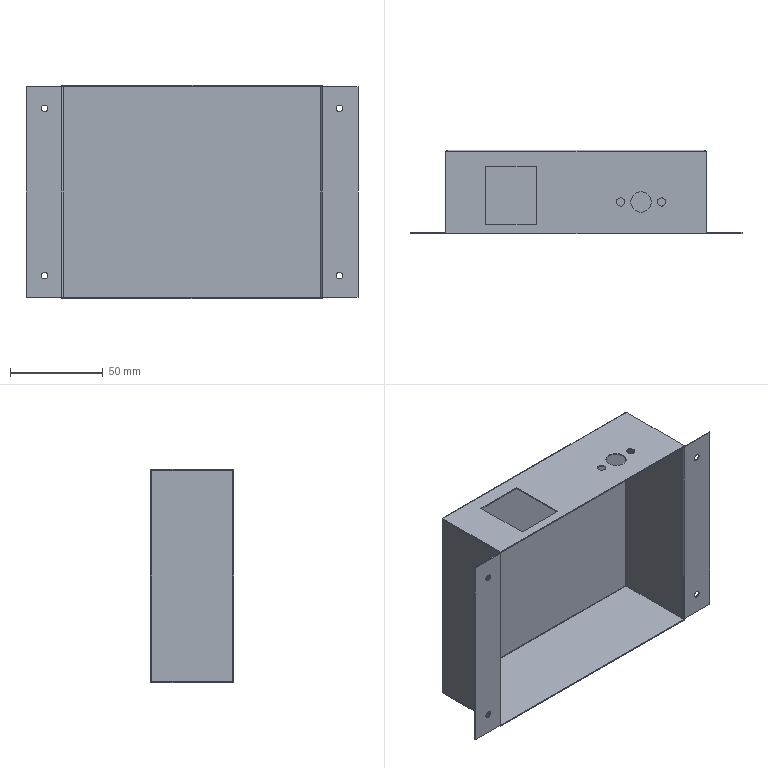Part | SolidWorks | features BaseBody 1 | 1 solid | 60 faces | box 178.6 x 44.9 x 114.8 mm | volume 25020 mm3 | plane 30 | cylinder 26 | spline 4 | commonest cylinder face diameters 3.5 x8 0.4 x6 1.6 x6 4.5 x4 11 x2